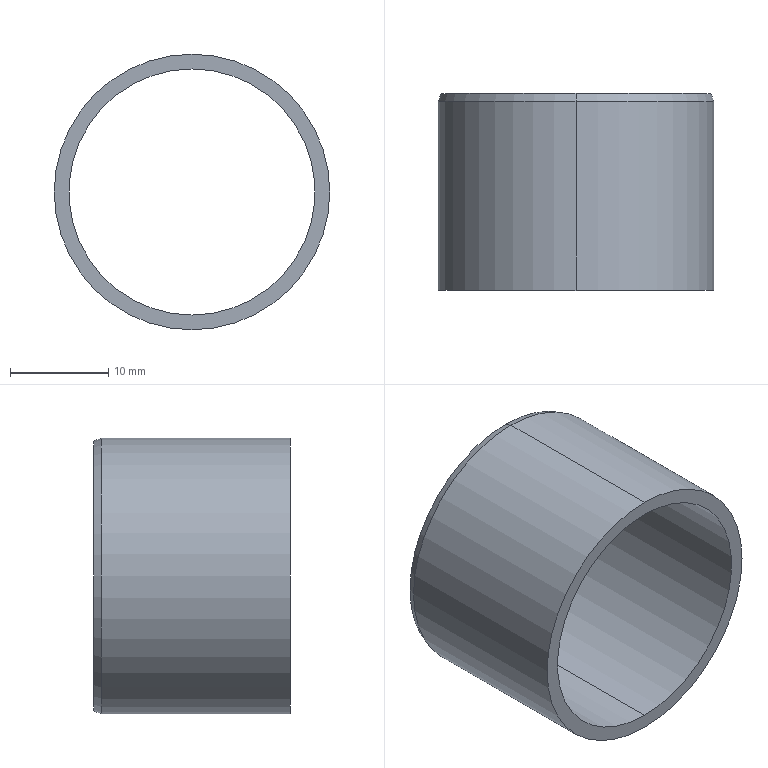Part | STEP file | PN_0016_default | 1 solid | 8 faces | box 28 x 20 x 28 mm | volume 2487 mm3 | cylinder 4 | cone 2 | plane 2 | commonest cylinder face diameters 25 x2 28 x2
STEP:
#1=CARTESIAN_POINT('',(0.,0.,0.));
#2=DIRECTION('',(0.,0.,1.));
#3=DIRECTION('',(1.,0.,0.));
#4=AXIS2_PLACEMENT_3D('',#1,#2,#3);
#5=CARTESIAN_POINT('',(0.,0.,12.5));
#6=VERTEX_POINT('',#5);
#7=CARTESIAN_POINT('',(0.,20.,12.5));
#8=VERTEX_POINT('',#7);
#9=CARTESIAN_POINT('',(0.,0.,12.5));
#10=DIRECTION('',(0.,1.,0.));
#11=VECTOR('',#10,1.);
#12=LINE('',#9,#11);
#13=CARTESIAN_POINT('',(0.,0.,0.));
#14=DIRECTION('',(0.,1.,0.));
#15=DIRECTION('',(0.,0.,1.));
#16=AXIS2_PLACEMENT_3D('',#13,#14,#15);
#17=CYLINDRICAL_SURFACE('',#16,12.5);
#18=CARTESIAN_POINT('',(6.283,0.));
#19=DIRECTION('',(0.,1.));
#20=VECTOR('',#19,1.);
#21=LINE('',#18,#20);
#22=(GEOMETRIC_REPRESENTATION_CONTEXT(2)PARAMETRIC_REPRESENTATION_CONTEXT()REPRESENTATION_CONTEXT('',''));
#23=DEFINITIONAL_REPRESENTATION('',(#21),#22);
#24=PCURVE('',#17,#23);
#25=CARTESIAN_POINT('',(0.,0.,0.));
#26=DIRECTION('',(0.,1.,0.));
#27=DIRECTION('',(0.,0.,1.));
#28=AXIS2_PLACEMENT_3D('',#25,#26,#27);
#29=CYLINDRICAL_SURFACE('',#28,12.5);
#30=CARTESIAN_POINT('',(0.,0.));
#31=DIRECTION('',(0.,1.));
#32=VECTOR('',#31,1.);
#33=LINE('',#30,#32);
#34=(GEOMETRIC_REPRESENTATION_CONTEXT(2)PARAMETRIC_REPRESENTATION_CONTEXT()REPRESENTATION_CONTEXT('',''));
#35=DEFINITIONAL_REPRESENTATION('',(#33),#34);
#36=PCURVE('',#29,#35);
#37=SURFACE_CURVE('',#12,(#24,#36),.PCURVE_S1.);
#38=EDGE_CURVE('',#6,#8,#37,.T.);
#39=ORIENTED_EDGE('',*,*,#38,.T.);
#40=CARTESIAN_POINT('',(0.,20.,-12.5));
#41=VERTEX_POINT('',#40);
#42=CARTESIAN_POINT('',(0.,20.,0.));
#43=DIRECTION('',(0.,1.,0.));
#44=DIRECTION('',(0.,0.,1.));
#45=AXIS2_PLACEMENT_3D('',#42,#43,#44);
#46=CIRCLE('',#45,12.5);
#47=CARTESIAN_POINT('',(0.,20.));
#48=DIRECTION('',(1.,0.));
#49=VECTOR('',#48,1.);
#50=LINE('',#47,#49);
#51=(GEOMETRIC_REPRESENTATION_CONTEXT(2)PARAMETRIC_REPRESENTATION_CONTEXT()REPRESENTATION_CONTEXT('',''));
#52=DEFINITIONAL_REPRESENTATION('',(#50),#51);
#53=PCURVE('',#17,#52);
#54=CARTESIAN_POINT('',(13.709,20.,0.));
#55=DIRECTION('',(0.,-1.,0.));
#56=DIRECTION('',(0.,0.,-1.));
#57=AXIS2_PLACEMENT_3D('',#54,#55,#56);
#58=PLANE('',#57);
#59=CARTESIAN_POINT('',(-12.5,-13.709));
#60=CARTESIAN_POINT('',(-12.5,7.942));
#61=CARTESIAN_POINT('',(6.25,-2.884));
#62=CARTESIAN_POINT('',(25.,-13.709));
#63=CARTESIAN_POINT('',(6.25,-24.534));
#64=CARTESIAN_POINT('',(-12.5,-35.359));
#65=CARTESIAN_POINT('',(-12.5,-13.709));
#66=(BOUNDED_CURVE()B_SPLINE_CURVE(2,(#59,#60,#61,#62,#63,#64,#65),.UNSPECIFIED.,.T.,.F.)B_SPLINE_CURVE_WITH_KNOTS((1,2,2,2,2,1),(-2.094,0.,2.094,4.189,6.283,8.378),.UNSPECIFIED.)CURVE()GEOMETRIC_REPRESENTATION_ITEM()RATIONAL_B_SPLINE_CURVE((1.,0.5,1.,0.5,1.,0.5,1.))REPRESENTATION_ITEM(''));
#67=(GEOMETRIC_REPRESENTATION_CONTEXT(2)PARAMETRIC_REPRESENTATION_CONTEXT()REPRESENTATION_CONTEXT('',''));
#68=DEFINITIONAL_REPRESENTATION('',(#66),#67);
#69=PCURVE('',#58,#68);
#70=SURFACE_CURVE('',#46,(#53,#69),.PCURVE_S1.);
#71=EDGE_CURVE('',#41,#8,#70,.T.);
#72=ORIENTED_EDGE('',*,*,#71,.F.);
#73=CARTESIAN_POINT('',(0.,0.,-12.5));
#74=VERTEX_POINT('',#73);
#75=CARTESIAN_POINT('',(0.,0.,-12.5));
#76=DIRECTION('',(0.,1.,0.));
#77=VECTOR('',#76,1.);
#78=LINE('',#75,#77);
#79=CARTESIAN_POINT('',(3.142,0.));
#80=DIRECTION('',(0.,1.));
#81=VECTOR('',#80,1.);
#82=LINE('',#79,#81);
#83=(GEOMETRIC_REPRESENTATION_CONTEXT(2)PARAMETRIC_REPRESENTATION_CONTEXT()REPRESENTATION_CONTEXT('',''));
#84=DEFINITIONAL_REPRESENTATION('',(#82),#83);
#85=PCURVE('',#17,#84);
#86=CARTESIAN_POINT('',(3.142,0.));
#87=DIRECTION('',(0.,1.));
#88=VECTOR('',#87,1.);
#89=LINE('',#86,#88);
#90=(GEOMETRIC_REPRESENTATION_CONTEXT(2)PARAMETRIC_REPRESENTATION_CONTEXT()REPRESENTATION_CONTEXT('',''));
#91=DEFINITIONAL_REPRESENTATION('',(#89),#90);
#92=PCURVE('',#29,#91);
#93=SURFACE_CURVE('',#78,(#85,#92),.PCURVE_S1.);
#94=EDGE_CURVE('',#74,#41,#93,.T.);
#95=ORIENTED_EDGE('',*,*,#94,.F.);
#96=CARTESIAN_POINT('',(0.,0.,0.));
#97=DIRECTION('',(0.,1.,0.));
#98=DIRECTION('',(0.,0.,1.));
#99=AXIS2_PLACEMENT_3D('',#96,#97,#98);
#100=CIRCLE('',#99,12.5);
#101=CARTESIAN_POINT('',(0.,0.));
#102=DIRECTION('',(1.,0.));
#103=VECTOR('',#102,1.);
#104=LINE('',#101,#103);
#105=(GEOMETRIC_REPRESENTATION_CONTEXT(2)PARAMETRIC_REPRESENTATION_CONTEXT()REPRESENTATION_CONTEXT('',''));
#106=DEFINITIONAL_REPRESENTATION('',(#104),#105);
#107=PCURVE('',#17,#106);
#108=CARTESIAN_POINT('',(12.5,0.,0.));
#109=DIRECTION('',(0.,1.,0.));
#110=DIRECTION('',(0.,0.,1.));
#111=AXIS2_PLACEMENT_3D('',#108,#109,#110);
#112=PLANE('',#111);
#113=CARTESIAN_POINT('',(0.,-12.5));
#114=DIRECTION('',(1.,0.));
#115=AXIS2_PLACEMENT_2D('',#113,#114);
#116=CIRCLE('',#115,12.5);
#117=(GEOMETRIC_REPRESENTATION_CONTEXT(2)PARAMETRIC_REPRESENTATION_CONTEXT()REPRESENTATION_CONTEXT('',''));
#118=DEFINITIONAL_REPRESENTATION('',(#116),#117);
#119=PCURVE('',#112,#118);
#120=SURFACE_CURVE('',#100,(#107,#119),.PCURVE_S1.);
#121=EDGE_CURVE('',#74,#6,#120,.T.);
#122=ORIENTED_EDGE('',*,*,#121,.T.);
#123=EDGE_LOOP('',(#39,#72,#95,#122));
#124=FACE_BOUND('',#123,.F.);
#125=ADVANCED_FACE('',(#124),#17,.F.);
#126=CARTESIAN_POINT('',(0.,20.,13.709));
#127=VERTEX_POINT('',#126);
#128=CARTESIAN_POINT('',(0.,20.,-13.709));
#129=VERTEX_POINT('',#128);
#130=CARTESIAN_POINT('',(0.,20.,0.));
#131=DIRECTION('',(0.,1.,0.));
#132=DIRECTION('',(0.,0.,1.));
#133=AXIS2_PLACEMENT_3D('',#130,#131,#132);
#134=CIRCLE('',#133,13.709);
#135=CARTESIAN_POINT('',(0.,19.2,0.));
#136=DIRECTION('',(0.,-1.,0.));
#137=DIRECTION('',(0.,0.,-1.));
#138=AXIS2_PLACEMENT_3D('',#135,#136,#137);
#139=CONICAL_SURFACE('',#138,14.,0.3491);
#140=CARTESIAN_POINT('',(3.142,-0.8));
#141=DIRECTION('',(-1.,0.));
#142=VECTOR('',#141,1.);
#143=LINE('',#140,#142);
#144=(GEOMETRIC_REPRESENTATION_CONTEXT(2)PARAMETRIC_REPRESENTATION_CONTEXT()REPRESENTATION_CONTEXT('',''));
#145=DEFINITIONAL_REPRESENTATION('',(#143),#144);
#146=PCURVE('',#139,#145);
#147=CARTESIAN_POINT('',(-13.709,-13.709));
#148=CARTESIAN_POINT('',(-13.709,10.036));
#149=CARTESIAN_POINT('',(6.854,-1.837));
#150=CARTESIAN_POINT('',(27.418,-13.709));
#151=CARTESIAN_POINT('',(6.854,-25.581));
#152=CARTESIAN_POINT('',(-13.709,-37.453));
#153=CARTESIAN_POINT('',(-13.709,-13.709));
#154=(BOUNDED_CURVE()B_SPLINE_CURVE(2,(#147,#148,#149,#150,#151,#152,#153),.UNSPECIFIED.,.T.,.F.)B_SPLINE_CURVE_WITH_KNOTS((1,2,2,2,2,1),(-2.094,0.,2.094,4.189,6.283,8.378),.UNSPECIFIED.)CURVE()GEOMETRIC_REPRESENTATION_ITEM()RATIONAL_B_SPLINE_CURVE((1.,0.5,1.,0.5,1.,0.5,1.))REPRESENTATION_ITEM(''));
#155=(GEOMETRIC_REPRESENTATION_CONTEXT(2)PARAMETRIC_REPRESENTATION_CONTEXT()REPRESENTATION_CONTEXT('',''));
#156=DEFINITIONAL_REPRESENTATION('',(#154),#155);
#157=PCURVE('',#58,#156);
#158=SURFACE_CURVE('',#134,(#146,#157),.PCURVE_S1.);
#159=EDGE_CURVE('',#127,#129,#158,.T.);
#160=ORIENTED_EDGE('',*,*,#159,.F.);
#161=CARTESIAN_POINT('',(0.,19.2,14.));
#162=VERTEX_POINT('',#161);
#163=CARTESIAN_POINT('',(0.,19.2,14.));
#164=DIRECTION('',(0.,-0.9397,0.342));
#165=VECTOR('',#164,1.);
#166=LINE('',#163,#165);
#167=CARTESIAN_POINT('',(3.142,0.));
#168=DIRECTION('',(0.,1.));
#169=VECTOR('',#168,1.);
#170=LINE('',#167,#169);
#171=(GEOMETRIC_REPRESENTATION_CONTEXT(2)PARAMETRIC_REPRESENTATION_CONTEXT()REPRESENTATION_CONTEXT('',''));
#172=DEFINITIONAL_REPRESENTATION('',(#170),#171);
#173=PCURVE('',#139,#172);
#174=CARTESIAN_POINT('',(0.,19.2,0.));
#175=DIRECTION('',(0.,-1.,0.));
#176=DIRECTION('',(0.,0.,-1.));
#177=AXIS2_PLACEMENT_3D('',#174,#175,#176);
#178=CONICAL_SURFACE('',#177,14.,0.3491);
#179=CARTESIAN_POINT('',(3.142,0.));
#180=DIRECTION('',(0.,1.));
#181=VECTOR('',#180,1.);
#182=LINE('',#179,#181);
#183=(GEOMETRIC_REPRESENTATION_CONTEXT(2)PARAMETRIC_REPRESENTATION_CONTEXT()REPRESENTATION_CONTEXT('',''));
#184=DEFINITIONAL_REPRESENTATION('',(#182),#183);
#185=PCURVE('',#178,#184);
#186=SURFACE_CURVE('',#166,(#173,#185),.PCURVE_S1.);
#187=EDGE_CURVE('',#127,#162,#186,.T.);
#188=ORIENTED_EDGE('',*,*,#187,.T.);
#189=CARTESIAN_POINT('',(0.,19.2,-14.));
#190=VERTEX_POINT('',#189);
#191=CARTESIAN_POINT('',(0.,19.2,0.));
#192=DIRECTION('',(0.,1.,0.));
#193=DIRECTION('',(0.,0.,1.));
#194=AXIS2_PLACEMENT_3D('',#191,#192,#193);
#195=CIRCLE('',#194,14.);
#196=CARTESIAN_POINT('',(3.142,0.));
#197=DIRECTION('',(-1.,0.));
#198=VECTOR('',#197,1.);
#199=LINE('',#196,#198);
#200=(GEOMETRIC_REPRESENTATION_CONTEXT(2)PARAMETRIC_REPRESENTATION_CONTEXT()REPRESENTATION_CONTEXT('',''));
#201=DEFINITIONAL_REPRESENTATION('',(#199),#200);
#202=PCURVE('',#139,#201);
#203=CARTESIAN_POINT('',(0.,0.,0.));
#204=DIRECTION('',(0.,1.,0.));
#205=DIRECTION('',(0.,0.,1.));
#206=AXIS2_PLACEMENT_3D('',#203,#204,#205);
#207=CYLINDRICAL_SURFACE('',#206,14.);
#208=CARTESIAN_POINT('',(0.,19.2));
#209=DIRECTION('',(1.,0.));
#210=VECTOR('',#209,1.);
#211=LINE('',#208,#210);
#212=(GEOMETRIC_REPRESENTATION_CONTEXT(2)PARAMETRIC_REPRESENTATION_CONTEXT()REPRESENTATION_CONTEXT('',''));
#213=DEFINITIONAL_REPRESENTATION('',(#211),#212);
#214=PCURVE('',#207,#213);
#215=SURFACE_CURVE('',#195,(#202,#214),.PCURVE_S1.);
#216=EDGE_CURVE('',#162,#190,#215,.T.);
#217=ORIENTED_EDGE('',*,*,#216,.T.);
#218=CARTESIAN_POINT('',(0.,19.2,-14.));
#219=DIRECTION('',(0.,-0.9397,-0.342));
#220=VECTOR('',#219,1.);
#221=LINE('',#218,#220);
#222=CARTESIAN_POINT('',(0.,0.));
#223=DIRECTION('',(0.,1.));
#224=VECTOR('',#223,1.);
#225=LINE('',#222,#224);
#226=(GEOMETRIC_REPRESENTATION_CONTEXT(2)PARAMETRIC_REPRESENTATION_CONTEXT()REPRESENTATION_CONTEXT('',''));
#227=DEFINITIONAL_REPRESENTATION('',(#225),#226);
#228=PCURVE('',#139,#227);
#229=CARTESIAN_POINT('',(6.283,0.));
#230=DIRECTION('',(0.,1.));
#231=VECTOR('',#230,1.);
#232=LINE('',#229,#231);
#233=(GEOMETRIC_REPRESENTATION_CONTEXT(2)PARAMETRIC_REPRESENTATION_CONTEXT()REPRESENTATION_CONTEXT('',''));
#234=DEFINITIONAL_REPRESENTATION('',(#232),#233);
#235=PCURVE('',#178,#234);
#236=SURFACE_CURVE('',#221,(#228,#235),.PCURVE_S1.);
#237=EDGE_CURVE('',#129,#190,#236,.T.);
#238=ORIENTED_EDGE('',*,*,#237,.F.);
#239=EDGE_LOOP('',(#160,#188,#217,#238));
#240=FACE_BOUND('',#239,.T.);
#241=ADVANCED_FACE('',(#240),#139,.T.);
#242=CARTESIAN_POINT('',(0.,0.,14.));
#243=VERTEX_POINT('',#242);
#244=CARTESIAN_POINT('',(0.,0.,-14.));
#245=VERTEX_POINT('',#244);
#246=CARTESIAN_POINT('',(0.,0.,0.));
#247=DIRECTION('',(0.,1.,0.));
#248=DIRECTION('',(0.,0.,1.));
#249=AXIS2_PLACEMENT_3D('',#246,#247,#248);
#250=CIRCLE('',#249,14.);
#251=CARTESIAN_POINT('',(0.,0.));
#252=DIRECTION('',(1.,0.));
#253=VECTOR('',#252,1.);
#254=LINE('',#251,#253);
#255=(GEOMETRIC_REPRESENTATION_CONTEXT(2)PARAMETRIC_REPRESENTATION_CONTEXT()REPRESENTATION_CONTEXT('',''));
#256=DEFINITIONAL_REPRESENTATION('',(#254),#255);
#257=PCURVE('',#207,#256);
#258=CARTESIAN_POINT('',(0.,-12.5));
#259=DIRECTION('',(1.,0.));
#260=AXIS2_PLACEMENT_2D('',#258,#259);
#261=CIRCLE('',#260,14.);
#262=(GEOMETRIC_REPRESENTATION_CONTEXT(2)PARAMETRIC_REPRESENTATION_CONTEXT()REPRESENTATION_CONTEXT('',''));
#263=DEFINITIONAL_REPRESENTATION('',(#261),#262);
#264=PCURVE('',#112,#263);
#265=SURFACE_CURVE('',#250,(#257,#264),.PCURVE_S1.);
#266=EDGE_CURVE('',#243,#245,#265,.T.);
#267=ORIENTED_EDGE('',*,*,#266,.T.);
#268=CARTESIAN_POINT('',(0.,0.,-14.));
#269=DIRECTION('',(0.,1.,0.));
#270=VECTOR('',#269,1.);
#271=LINE('',#268,#270);
#272=CARTESIAN_POINT('',(3.142,0.));
#273=DIRECTION('',(0.,1.));
#274=VECTOR('',#273,1.);
#275=LINE('',#272,#274);
#276=(GEOMETRIC_REPRESENTATION_CONTEXT(2)PARAMETRIC_REPRESENTATION_CONTEXT()REPRESENTATION_CONTEXT('',''));
#277=DEFINITIONAL_REPRESENTATION('',(#275),#276);
#278=PCURVE('',#207,#277);
#279=CARTESIAN_POINT('',(0.,0.,0.));
#280=DIRECTION('',(0.,1.,0.));
#281=DIRECTION('',(0.,0.,1.));
#282=AXIS2_PLACEMENT_3D('',#279,#280,#281);
#283=CYLINDRICAL_SURFACE('',#282,14.);
#284=CARTESIAN_POINT('',(3.142,0.));
#285=DIRECTION('',(0.,1.));
#286=VECTOR('',#285,1.);
#287=LINE('',#284,#286);
#288=(GEOMETRIC_REPRESENTATION_CONTEXT(2)PARAMETRIC_REPRESENTATION_CONTEXT()REPRESENTATION_CONTEXT('',''));
#289=DEFINITIONAL_REPRESENTATION('',(#287),#288);
#290=PCURVE('',#283,#289);
#291=SURFACE_CURVE('',#271,(#278,#290),.PCURVE_S1.);
#292=EDGE_CURVE('',#245,#190,#291,.T.);
#293=ORIENTED_EDGE('',*,*,#292,.T.);
#294=ORIENTED_EDGE('',*,*,#216,.F.);
#295=CARTESIAN_POINT('',(0.,0.,14.));
#296=DIRECTION('',(0.,1.,0.));
#297=VECTOR('',#296,1.);
#298=LINE('',#295,#297);
#299=CARTESIAN_POINT('',(0.,0.));
#300=DIRECTION('',(0.,1.));
#301=VECTOR('',#300,1.);
#302=LINE('',#299,#301);
#303=(GEOMETRIC_REPRESENTATION_CONTEXT(2)PARAMETRIC_REPRESENTATION_CONTEXT()REPRESENTATION_CONTEXT('',''));
#304=DEFINITIONAL_REPRESENTATION('',(#302),#303);
#305=PCURVE('',#207,#304);
#306=CARTESIAN_POINT('',(6.283,0.));
#307=DIRECTION('',(0.,1.));
#308=VECTOR('',#307,1.);
#309=LINE('',#306,#308);
#310=(GEOMETRIC_REPRESENTATION_CONTEXT(2)PARAMETRIC_REPRESENTATION_CONTEXT()REPRESENTATION_CONTEXT('',''));
#311=DEFINITIONAL_REPRESENTATION('',(#309),#310);
#312=PCURVE('',#283,#311);
#313=SURFACE_CURVE('',#298,(#305,#312),.PCURVE_S1.);
#314=EDGE_CURVE('',#243,#162,#313,.T.);
#315=ORIENTED_EDGE('',*,*,#314,.F.);
#316=EDGE_LOOP('',(#267,#293,#294,#315));
#317=FACE_BOUND('',#316,.T.);
#318=ADVANCED_FACE('',(#317),#207,.T.);
#319=ORIENTED_EDGE('',*,*,#266,.F.);
#320=CARTESIAN_POINT('',(0.,0.,0.));
#321=DIRECTION('',(0.,1.,0.));
#322=DIRECTION('',(0.,0.,1.));
#323=AXIS2_PLACEMENT_3D('',#320,#321,#322);
#324=CIRCLE('',#323,14.);
#325=CARTESIAN_POINT('',(0.,-12.5));
#326=DIRECTION('',(1.,0.));
#327=AXIS2_PLACEMENT_2D('',#325,#326);
#328=CIRCLE('',#327,14.);
#329=(GEOMETRIC_REPRESENTATION_CONTEXT(2)PARAMETRIC_REPRESENTATION_CONTEXT()REPRESENTATION_CONTEXT('',''));
#330=DEFINITIONAL_REPRESENTATION('',(#328),#329);
#331=PCURVE('',#112,#330);
#332=CARTESIAN_POINT('',(0.,0.));
#333=DIRECTION('',(1.,0.));
#334=VECTOR('',#333,1.);
#335=LINE('',#332,#334);
#336=(GEOMETRIC_REPRESENTATION_CONTEXT(2)PARAMETRIC_REPRESENTATION_CONTEXT()REPRESENTATION_CONTEXT('',''));
#337=DEFINITIONAL_REPRESENTATION('',(#335),#336);
#338=PCURVE('',#283,#337);
#339=SURFACE_CURVE('',#324,(#331,#338),.PCURVE_S1.);
#340=EDGE_CURVE('',#245,#243,#339,.T.);
#341=ORIENTED_EDGE('',*,*,#340,.F.);
#342=EDGE_LOOP('',(#319,#341));
#343=FACE_BOUND('',#342,.T.);
#344=CARTESIAN_POINT('',(0.,0.,0.));
#345=DIRECTION('',(0.,1.,0.));
#346=DIRECTION('',(0.,0.,1.));
#347=AXIS2_PLACEMENT_3D('',#344,#345,#346);
#348=CIRCLE('',#347,12.5);
#349=CARTESIAN_POINT('',(0.,-12.5));
#350=DIRECTION('',(1.,0.));
#351=AXIS2_PLACEMENT_2D('',#349,#350);
#352=CIRCLE('',#351,12.5);
#353=(GEOMETRIC_REPRESENTATION_CONTEXT(2)PARAMETRIC_REPRESENTATION_CONTEXT()REPRESENTATION_CONTEXT('',''));
#354=DEFINITIONAL_REPRESENTATION('',(#352),#353);
#355=PCURVE('',#112,#354);
#356=CARTESIAN_POINT('',(0.,0.));
#357=DIRECTION('',(1.,0.));
#358=VECTOR('',#357,1.);
#359=LINE('',#356,#358);
#360=(GEOMETRIC_REPRESENTATION_CONTEXT(2)PARAMETRIC_REPRESENTATION_CONTEXT()REPRESENTATION_CONTEXT('',''));
#361=DEFINITIONAL_REPRESENTATION('',(#359),#360);
#362=PCURVE('',#29,#361);
#363=SURFACE_CURVE('',#348,(#355,#362),.PCURVE_S1.);
#364=EDGE_CURVE('',#6,#74,#363,.T.);
#365=ORIENTED_EDGE('',*,*,#364,.T.);
#366=ORIENTED_EDGE('',*,*,#121,.T.);
#367=EDGE_LOOP('',(#365,#366));
#368=FACE_BOUND('',#367,.T.);
#369=ADVANCED_FACE('',(#343,#368),#112,.F.);
#370=ORIENTED_EDGE('',*,*,#292,.F.);
#371=ORIENTED_EDGE('',*,*,#340,.T.);
#372=ORIENTED_EDGE('',*,*,#314,.T.);
#373=CARTESIAN_POINT('',(0.,19.2,0.));
#374=DIRECTION('',(0.,1.,0.));
#375=DIRECTION('',(0.,0.,1.));
#376=AXIS2_PLACEMENT_3D('',#373,#374,#375);
#377=CIRCLE('',#376,14.);
#378=CARTESIAN_POINT('',(0.,19.2));
#379=DIRECTION('',(1.,0.));
#380=VECTOR('',#379,1.);
#381=LINE('',#378,#380);
#382=(GEOMETRIC_REPRESENTATION_CONTEXT(2)PARAMETRIC_REPRESENTATION_CONTEXT()REPRESENTATION_CONTEXT('',''));
#383=DEFINITIONAL_REPRESENTATION('',(#381),#382);
#384=PCURVE('',#283,#383);
#385=CARTESIAN_POINT('',(9.425,0.));
#386=DIRECTION('',(-1.,0.));
#387=VECTOR('',#386,1.);
#388=LINE('',#385,#387);
#389=(GEOMETRIC_REPRESENTATION_CONTEXT(2)PARAMETRIC_REPRESENTATION_CONTEXT()REPRESENTATION_CONTEXT('',''));
#390=DEFINITIONAL_REPRESENTATION('',(#388),#389);
#391=PCURVE('',#178,#390);
#392=SURFACE_CURVE('',#377,(#384,#391),.PCURVE_S1.);
#393=EDGE_CURVE('',#190,#162,#392,.T.);
#394=ORIENTED_EDGE('',*,*,#393,.F.);
#395=EDGE_LOOP('',(#370,#371,#372,#394));
#396=FACE_BOUND('',#395,.T.);
#397=ADVANCED_FACE('',(#396),#283,.T.);
#398=ORIENTED_EDGE('',*,*,#187,.F.);
#399=CARTESIAN_POINT('',(0.,20.,0.));
#400=DIRECTION('',(0.,1.,0.));
#401=DIRECTION('',(0.,0.,1.));
#402=AXIS2_PLACEMENT_3D('',#399,#400,#401);
#403=CIRCLE('',#402,13.709);
#404=CARTESIAN_POINT('',(9.425,-0.8));
#405=DIRECTION('',(-1.,0.));
#406=VECTOR('',#405,1.);
#407=LINE('',#404,#406);
#408=(GEOMETRIC_REPRESENTATION_CONTEXT(2)PARAMETRIC_REPRESENTATION_CONTEXT()REPRESENTATION_CONTEXT('',''));
#409=DEFINITIONAL_REPRESENTATION('',(#407),#408);
#410=PCURVE('',#178,#409);
#411=CARTESIAN_POINT('',(-13.709,-13.709));
#412=CARTESIAN_POINT('',(-13.709,10.036));
#413=CARTESIAN_POINT('',(6.854,-1.837));
#414=CARTESIAN_POINT('',(27.418,-13.709));
#415=CARTESIAN_POINT('',(6.854,-25.581));
#416=CARTESIAN_POINT('',(-13.709,-37.453));
#417=CARTESIAN_POINT('',(-13.709,-13.709));
#418=(BOUNDED_CURVE()B_SPLINE_CURVE(2,(#411,#412,#413,#414,#415,#416,#417),.UNSPECIFIED.,.T.,.F.)B_SPLINE_CURVE_WITH_KNOTS((1,2,2,2,2,1),(-2.094,0.,2.094,4.189,6.283,8.378),.UNSPECIFIED.)CURVE()GEOMETRIC_REPRESENTATION_ITEM()RATIONAL_B_SPLINE_CURVE((1.,0.5,1.,0.5,1.,0.5,1.))REPRESENTATION_ITEM(''));
#419=(GEOMETRIC_REPRESENTATION_CONTEXT(2)PARAMETRIC_REPRESENTATION_CONTEXT()REPRESENTATION_CONTEXT('',''));
#420=DEFINITIONAL_REPRESENTATION('',(#418),#419);
#421=PCURVE('',#58,#420);
#422=SURFACE_CURVE('',#403,(#410,#421),.PCURVE_S1.);
#423=EDGE_CURVE('',#129,#127,#422,.T.);
#424=ORIENTED_EDGE('',*,*,#423,.F.);
#425=ORIENTED_EDGE('',*,*,#237,.T.);
#426=ORIENTED_EDGE('',*,*,#393,.T.);
#427=EDGE_LOOP('',(#398,#424,#425,#426));
#428=FACE_BOUND('',#427,.T.);
#429=ADVANCED_FACE('',(#428),#178,.T.);
#430=CARTESIAN_POINT('',(0.,20.,0.));
#431=DIRECTION('',(0.,1.,0.));
#432=DIRECTION('',(0.,0.,1.));
#433=AXIS2_PLACEMENT_3D('',#430,#431,#432);
#434=CIRCLE('',#433,12.5);
#435=CARTESIAN_POINT('',(-12.5,-13.709));
#436=CARTESIAN_POINT('',(-12.5,7.942));
#437=CARTESIAN_POINT('',(6.25,-2.884));
#438=CARTESIAN_POINT('',(25.,-13.709));
#439=CARTESIAN_POINT('',(6.25,-24.534));
#440=CARTESIAN_POINT('',(-12.5,-35.359));
#441=CARTESIAN_POINT('',(-12.5,-13.709));
#442=(BOUNDED_CURVE()B_SPLINE_CURVE(2,(#435,#436,#437,#438,#439,#440,#441),.UNSPECIFIED.,.T.,.F.)B_SPLINE_CURVE_WITH_KNOTS((1,2,2,2,2,1),(-2.094,0.,2.094,4.189,6.283,8.378),.UNSPECIFIED.)CURVE()GEOMETRIC_REPRESENTATION_ITEM()RATIONAL_B_SPLINE_CURVE((1.,0.5,1.,0.5,1.,0.5,1.))REPRESENTATION_ITEM(''));
#443=(GEOMETRIC_REPRESENTATION_CONTEXT(2)PARAMETRIC_REPRESENTATION_CONTEXT()REPRESENTATION_CONTEXT('',''));
#444=DEFINITIONAL_REPRESENTATION('',(#442),#443);
#445=PCURVE('',#58,#444);
#446=CARTESIAN_POINT('',(0.,20.));
#447=DIRECTION('',(1.,0.));
#448=VECTOR('',#447,1.);
#449=LINE('',#446,#448);
#450=(GEOMETRIC_REPRESENTATION_CONTEXT(2)PARAMETRIC_REPRESENTATION_CONTEXT()REPRESENTATION_CONTEXT('',''));
#451=DEFINITIONAL_REPRESENTATION('',(#449),#450);
#452=PCURVE('',#29,#451);
#453=SURFACE_CURVE('',#434,(#445,#452),.PCURVE_S1.);
#454=EDGE_CURVE('',#8,#41,#453,.T.);
#455=ORIENTED_EDGE('',*,*,#454,.F.);
#456=ORIENTED_EDGE('',*,*,#71,.F.);
#457=EDGE_LOOP('',(#455,#456));
#458=FACE_BOUND('',#457,.T.);
#459=ORIENTED_EDGE('',*,*,#423,.T.);
#460=ORIENTED_EDGE('',*,*,#159,.T.);
#461=EDGE_LOOP('',(#459,#460));
#462=FACE_BOUND('',#461,.T.);
#463=ADVANCED_FACE('',(#458,#462),#58,.F.);
#464=ORIENTED_EDGE('',*,*,#454,.F.);
#465=ORIENTED_EDGE('',*,*,#38,.F.);
#466=ORIENTED_EDGE('',*,*,#364,.T.);
#467=ORIENTED_EDGE('',*,*,#94,.T.);
#468=EDGE_LOOP('',(#464,#465,#466,#467));
#469=FACE_BOUND('',#468,.F.);
#470=ADVANCED_FACE('',(#469),#29,.F.);
#471=CLOSED_SHELL('',(#125,#241,#318,#369,#397,#429,#463,#470));
#472=MANIFOLD_SOLID_BREP('',#471);
#473=(LENGTH_UNIT()NAMED_UNIT(*)SI_UNIT(.MILLI.,.METRE.));
#474=UNCERTAINTY_MEASURE_WITH_UNIT(LENGTH_MEASURE(0.0000001),#473,'','');
#475=(NAMED_UNIT(*)PLANE_ANGLE_UNIT()SI_UNIT($,.RADIAN.));
#476=(NAMED_UNIT(*)SI_UNIT($,.STERADIAN.)SOLID_ANGLE_UNIT());
#477=(GEOMETRIC_REPRESENTATION_CONTEXT(3)GLOBAL_UNCERTAINTY_ASSIGNED_CONTEXT((#474))GLOBAL_UNIT_ASSIGNED_CONTEXT((#473,#475,#476))REPRESENTATION_CONTEXT('',''));
#478=ADVANCED_BREP_SHAPE_REPRESENTATION('',(#4,#472),#477);